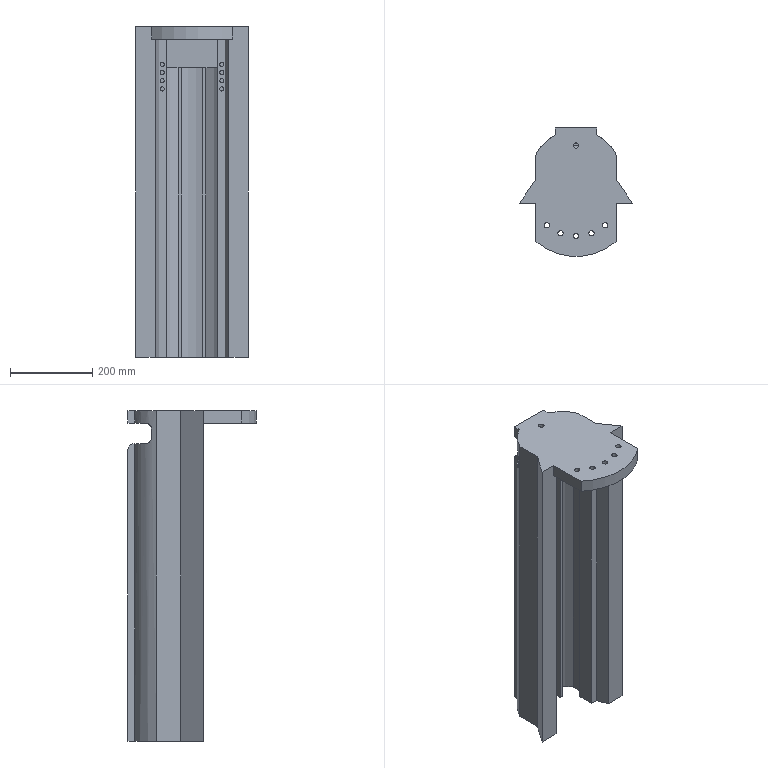Part | SolidWorks | features ICE 9, Fillet 2, Extrusion 1 | 1 solid | 105 faces | box 275.23 x 313.202 x 805 mm | volume 12308748 mm3 | plane 56 | cylinder 49 | commonest cylinder face diameters 10 x16 13 x12 26 x10 30 x3 180 x3 26.6 x2